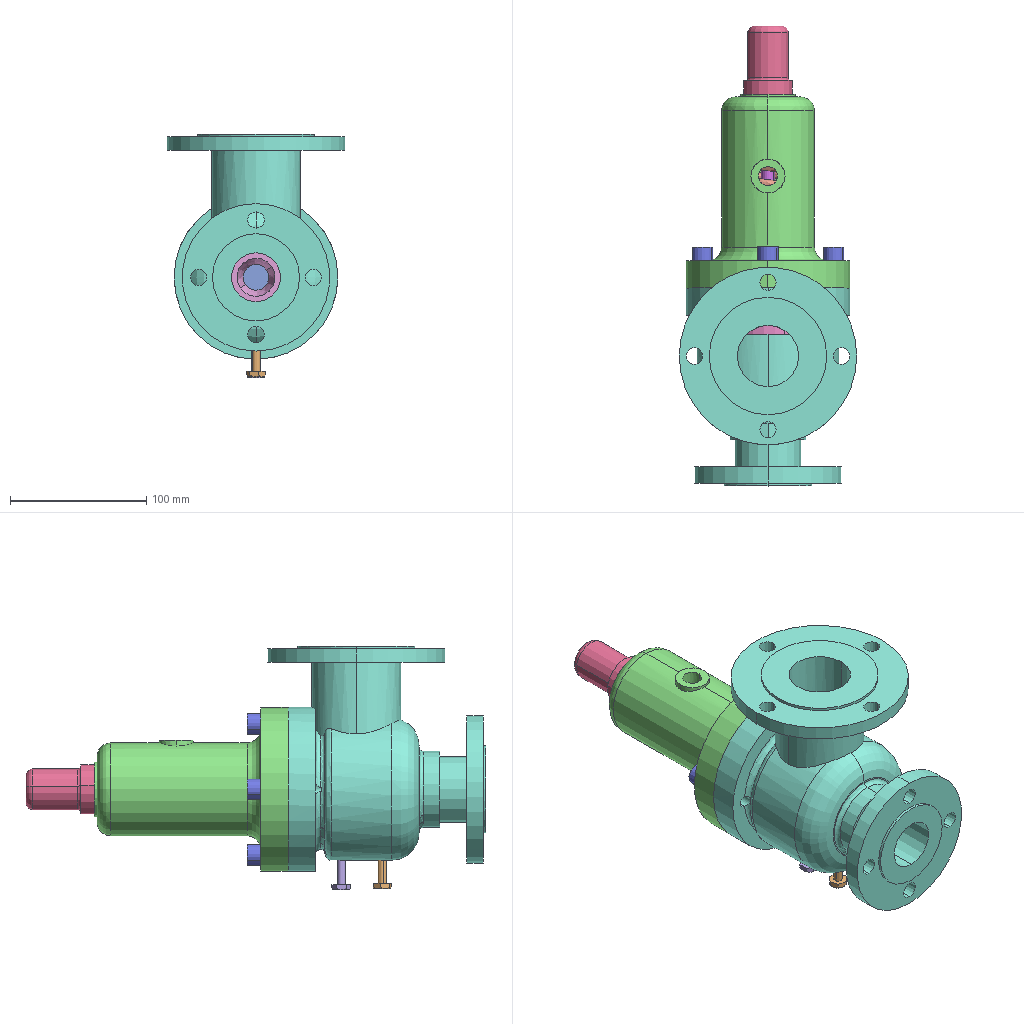Assembly | SolidWorks | 18 different items | 21 placed | box 130 x 337 x 179 mm
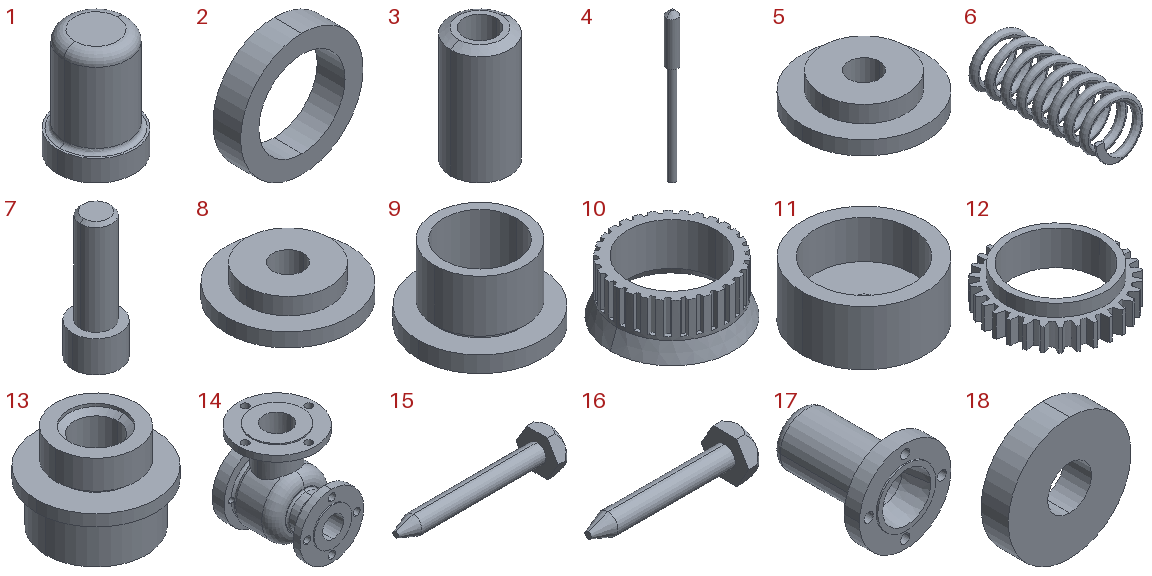Parts list (item | quantity | size | volume | features):
1 | x1 | 36 x 36 x 50 mm | 14046 mm3 | features HoleWzd 1, Revolution 1
2 | x1 | 22 x 5 x 22 mm | 957.204 mm3 | features Extrusion 1, HoleWzd 1
3 | x1 | 18 x 18 x 35 mm | 6065 mm3 | features Revolution 1
4 | x1 | 16 x 16 x 210 mm | 24181 mm3 | features Revolution 1
5 | x1 | 44 x 44 x 11 mm | 10654 mm3 | features Revolution 1
6 | x1 | 42 x 103.92 x 42 mm | 26599 mm3 | features Helix 1, ICE 1, Sweep 1
7 | x4 | 15 x 15 x 40 mm | 3707 mm3 | features ICE 3, Chamfer 1, Revolution 1
8 | x1 | 44 x 44 x 11 mm | 10654 mm3 | features Revolution 1
9 | x1 | 76 x 76 x 45 mm | 64785 mm3 | features Revolution 1
10 | x1 | 70.779 x 70.779 x 30 mm | 32307 mm3 | features CirPattern 1, HoleWzd 1, ICE 1, Revolution 1
11 | x1 | 45 x 45 x 20 mm | 18314 mm3 | features Revolution 1
12 | x1 | 50 x 49.844 x 14 mm | 8157 mm3 | features CirPattern 1, ICE 1, Revolution 1
13 | x1 | 52 x 52 x 38 mm | 38206 mm3 | features Revolution 1
14 | x1 | 130 x 160 x 165 mm | 638021 mm3 | features ICE 3, HoleWzd 2, Revolution 2, RevCut 1
15 | x1 | 51 x 13.856 x 12 mm | 1735 mm3 | features Extrusion 1, ICE 1, Revolution 1
16 | x1 | 44 x 13.856 x 12 mm | 1537 mm3 | features Extrusion 1, ICE 1, Revolution 1
17 | x1 | 120 x 152 x 120 mm | 371857 mm3 | features ICE 3, HoleWzd 1, Revolution 1
18 | x1 | 45 x 10 x 45 mm | 13894 mm3 | features Extrusion 1
Mates (type | each side: item.copy, entity, surface, feature):
Concentric | 13.1 edge | 14.1 edge
Coincident | 13.1 face plane Revolve1 | 14.1 face plane Cut-Revolve1
Concentric | 12.1 edge | 13.1 edge
Coincident | 12.1 face plane Revolve1 | 13.1 face plane Revolve1
Concentric | 11.1 edge | 13.1 edge
Coincident | 11.1 face plane Revolve1 | 12.1 face plane Revolve1
Concentric | 10.1 edge | 13.1 edge
Coincident | 10.1 face plane Revolve1 | 12.1 face plane Revolve1
Concentric | 11.1 edge | 18.1 edge
Coincident | 11.1 face plane Revolve1 | 18.1 face plane Boss-Extrude1
Concentric | 9.1 edge | 18.1 edge
Coincident | 14.1 face plane Cut-Revolve1 | 9.1 face plane Revolve1
Concentric | 14.1 edge | 17.1 edge
Concentric | 14.1 face cylinder M10 Tapped Hole1 | 17.1 face cylinder Cut-Extrude2
Coincident | 17.1 face plane Revolve1 | 9.1 face plane Revolve1
Concentric | 17.1 edge | 4.1 edge
Coincident | 11.1 edge | 4.1 edge
Concentric | 4.1 edge | 8.1 edge
Coincident | 4.1 face cone Revolve1 | 8.1 face cone Revolve1
Concentric | 6.1 select_type:24 | 8.1 edge
Coincident | 6.1 face plane Cut-Extrude2 | 8.1 face plane Revolve1
Concentric | 17.1 face cylinder M18x1.5 Tapped Hole1 | 5.1 edge
Coincident | 5.1 face plane Revolve1 | 6.1 face plane Cut-Extrude2
Concentric | 17.1 edge | 3.1 edge
Coincident | 3.1 face cone Revolve1 | 5.1 face cone Revolve1
Concentric | 2.1 edge | 3.1 edge
Coincident | 17.1 face plane Revolve1 | 2.1 face plane Boss-Extrude1
Concentric | 17.1 edge | 1.1 edge
Coincident | 17.1 face plane Revolve1 | 1.1 face plane Revolve1
Concentric | 14.1 face cylinder M6 Tapped Hole1 | 16.1 face cylinder Revolve1
Coincident | 10.1 face plane CirPattern1 | 16.1 edge
Concentric | 14.1 face cylinder M6 Tapped Hole1 | 15.1 face cylinder Revolve1
Tangent | 12.1 face cylinder CirPattern1 | 15.1 face plane Revolve1
Concentric | 17.1 face cylinder Cut-Extrude2 | 7.1 face cylinder Revolve1
Concentric | 17.1 face cylinder Cut-Extrude2 | 7.2 face cylinder Revolve1
Concentric | 17.1 face cylinder Cut-Extrude2 | 7.3 face cylinder Revolve1
Concentric | 17.1 face cylinder Cut-Extrude2 | 7.4 face cylinder Revolve1
Coincident | 17.1 face plane Revolve1 | 7.4 face plane Revolve1
Coincident | 17.1 face plane Revolve1 | 7.1 face plane Revolve1
Coincident | 17.1 face plane Revolve1 | 7.3 face plane Revolve1
Coincident | 17.1 face plane Revolve1 | 7.2 face plane Revolve1